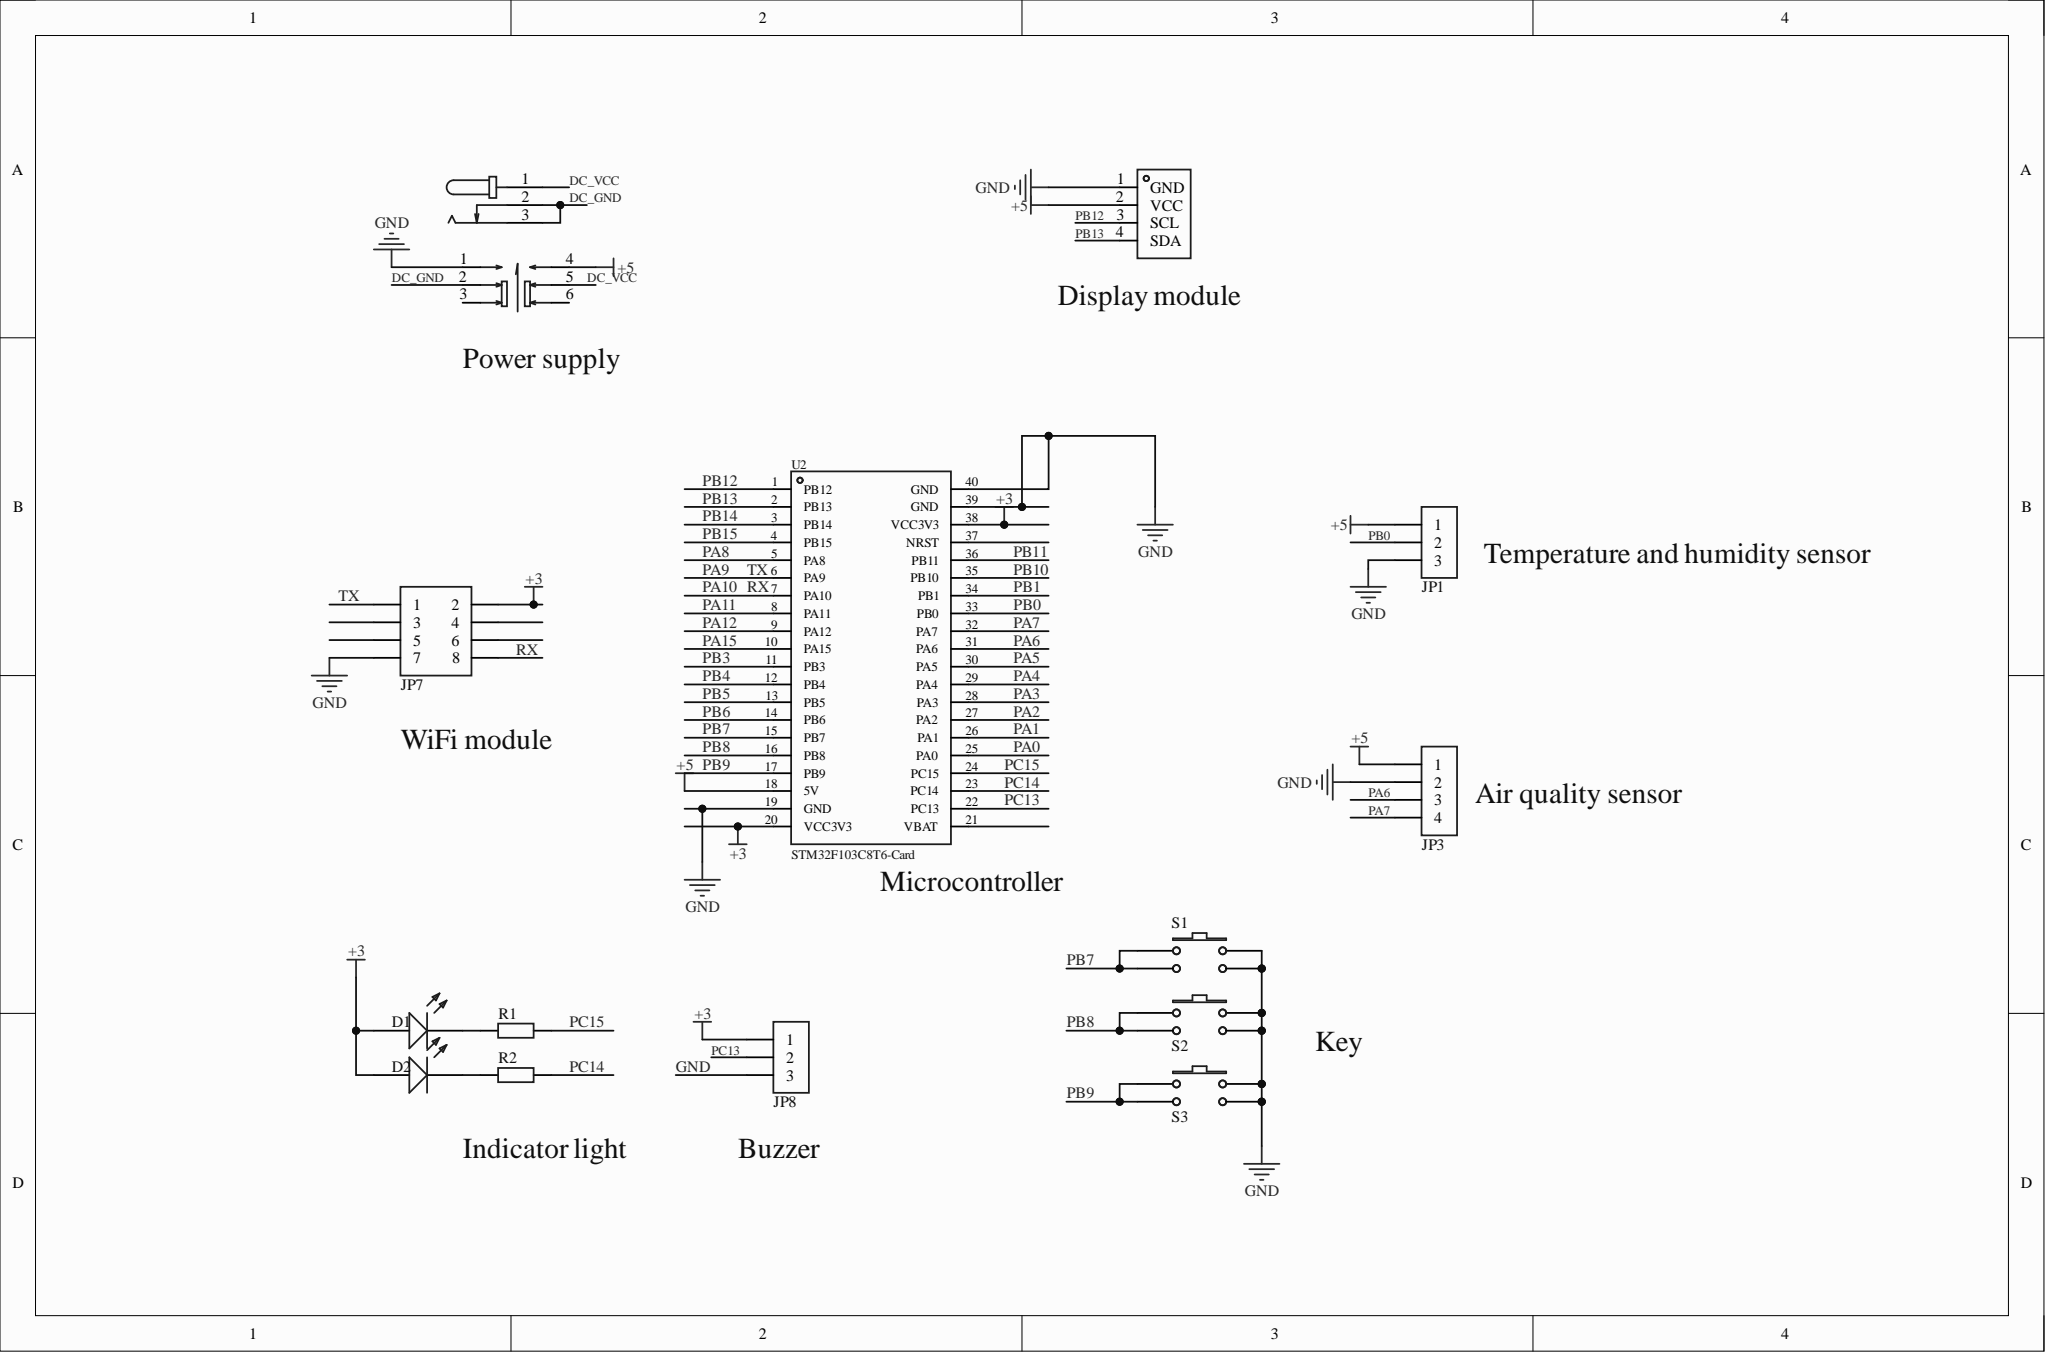Circuit board | Altium Designer | 15 parts | 20 nets
Bill of materials:
Comment,Description,Designator,Footprint,LibRef,Quantity
"led","","D1, D2","LED-TH_5mm","led","2"
"DC002-1.3","","DC1","DC-IN-TH_DC002-1.3","DC002-1.3","1"
"HDR-1X3","3P connector","JP1, JP8","HDR-TH_3P-P2.54-V-M-1","Header 3","2"
"HDR-1X4","4P connector","JP3","HDR-TH_4P-P2.54-V-M-1","Header 4","1"
"Header 4X2","4*2P connector","JP7","HDR-TH_8P-P2.54-V-F-R2-C4-S2.54-1","Header 4X2","1"
"Res2","Resistor","R1, R2","Res_1/8W","Res2","2"
"key_4","","S1, S2, S3","SW-TH_4P-L6.0-W6.0-P4.50-LS6.5","key_4","3"
"Self-lock button","","SW1","SW-TH_6P-L7.0-W7.0-P2.00","XKB7070-Z","1"
"OLED","","U1","OLED-TH_L27.8-W27.2-P2.54_C9900033791","OLED0.96","1"
"STM32F103C8T6-Card","","U2","CONN-TH_L53.3-W22.9_STM32F103C8T6-CARD","STM32F103C8T6-Card","1"
Netlist (Protel format):
[
D1
LED-TH_5mm
led



]
[
D2
LED-TH_5mm
led



]
[
DC1
DC-IN-TH_DC002-1.3
DC002-1.3



]
[
JP1
HDR-TH_3P-P2.54-V-M-1
HDR-1X3



]
[
JP3
HDR-TH_4P-P2.54-V-M-1
HDR-1X4



]
[
JP7
HDR-TH_8P-P2.54-V-F-R2-C4-S2.54-1
Header 4X2



]
[
JP8
HDR-TH_3P-P2.54-V-M-1
HDR-1X3



]
[
R1
Res_1/8W
Res2



]
[
R2
Res_1/8W
Res2



]
[
S1
SW-TH_4P-L6.0-W6.0-P4.50-LS6.5
key_4



]
[
S2
SW-TH_4P-L6.0-W6.0-P4.50-LS6.5
key_4



]
[
S3
SW-TH_4P-L6.0-W6.0-P4.50-LS6.5
key_4



]
[
SW1
SW-TH_6P-L7.0-W7.0-P2.00
Self-lock button



]
[
U1
OLED-TH_L27.8-W27.2-P2.54_C9900033791
OLED



]
[
U2
CONN-TH_L53.3-W22.9_STM32F103C8T6-CARD
STM32F103C8T6-Card



]
(
PC15
R1-2
U2-24
)
(
PC14
R2-2
U2-23
)
(
PC13
JP8-2
U2-22
)
(
PB13
U1-4
U2-2
)
(
PB12
U1-3
U2-1
)
(
PB9
S3-1
S3-3
U2-17
)
(
PB8
S2-1
S2-3
U2-16
)
(
PB7
S1-1
S1-3
U2-15
)
(
PB0
JP1-2
U2-33
)
(
PA10
JP7-8
U2-7
)
(
PA9
JP7-1
U2-6
)
(
PA7
JP3-4
U2-32
)
(
PA6
JP3-3
U2-31
)
(
NetD2_2
D2-2
R2-1
)
(
NetD1_2
D1-2
R1-1
)
(
GND
JP1-3
JP3-2
JP7-7
JP8-3
S1-2
S1-4
S2-2
S2-4
S3-2
S3-4
SW1-1
U1-1
U2-19
U2-39
U2-40
)
(
DC_VCC
DC1-1
SW1-5
)
(
DC_GND
DC1-2
DC1-3
SW1-2
)
(
+5
JP1-1
JP3-1
SW1-4
U1-2
U2-18
)
(
+3
D1-1
D2-1
JP7-2
JP8-1
U2-20
U2-38
)